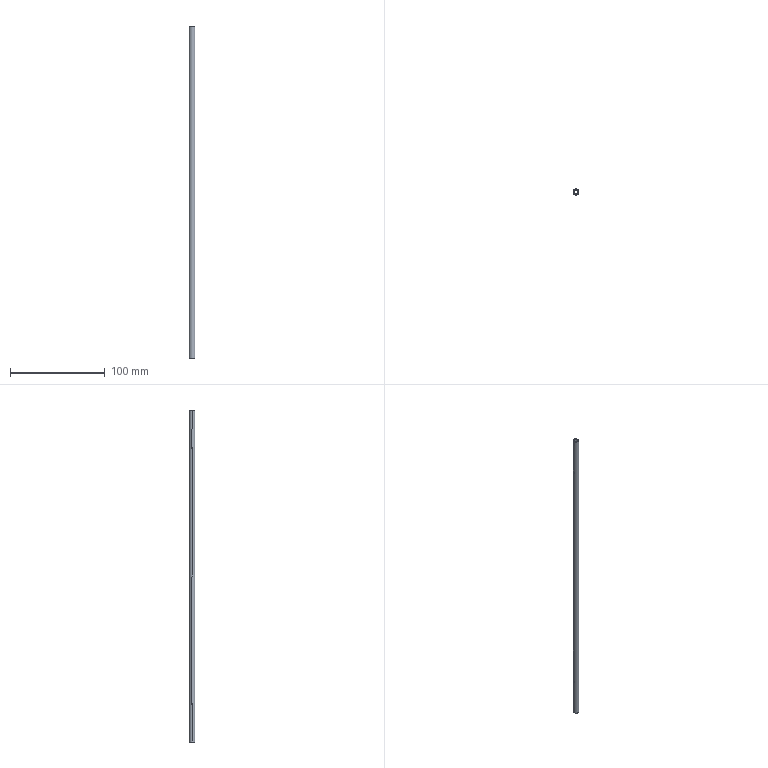Part | SolidWorks | features Extrusion 1, ICE 1 | 1 solid | 14 faces | box 6 x 6 x 350 mm | volume 5491 mm3 | cylinder 12 | plane 2 | commonest cylinder face diameters 1.5 x8 4 x2 6 x2
STEP:
#1=CARTESIAN_POINT('',(-2.,0.,310.75));
#2=VERTEX_POINT('',#1);
#3=CARTESIAN_POINT('',(-2.,0.,309.25));
#4=VERTEX_POINT('',#3);
#5=CARTESIAN_POINT('',(-2.,0.,310.75));
#6=CARTESIAN_POINT('',(-2.,-0.1001,310.75));
#7=CARTESIAN_POINT('',(-1.992,-0.1982,310.73));
#8=CARTESIAN_POINT('',(-1.966,-0.3796,310.654));
#9=CARTESIAN_POINT('',(-1.947,-0.4621,310.599));
#10=CARTESIAN_POINT('',(-1.909,-0.5991,310.461));
#11=CARTESIAN_POINT('',(-1.89,-0.6547,310.379));
#12=CARTESIAN_POINT('',(-1.863,-0.7298,310.199));
#13=CARTESIAN_POINT('',(-1.854,-0.7499,310.099));
#14=CARTESIAN_POINT('',(-1.854,-0.7501,309.902));
#15=CARTESIAN_POINT('',(-1.862,-0.7304,309.803));
#16=CARTESIAN_POINT('',(-1.89,-0.6542,309.62));
#17=CARTESIAN_POINT('',(-1.91,-0.5989,309.538));
#18=CARTESIAN_POINT('',(-1.947,-0.4613,309.401));
#19=CARTESIAN_POINT('',(-1.966,-0.3786,309.345));
#20=CARTESIAN_POINT('',(-1.992,-0.1981,309.27));
#21=CARTESIAN_POINT('',(-2.,-0.09859,309.25));
#22=CARTESIAN_POINT('',(-2.,0.,309.25));
#23=B_SPLINE_CURVE_WITH_KNOTS('',3,(#5,#6,#7,#8,#9,#10,#11,#12,#13,#14,#15,#16,#17,#18,#19,#20,#21,#22),.UNSPECIFIED.,.F.,.F.,(4,2,2,2,2,2,2,2,4),(0.,0.0002958,0.0005917,0.0008875,0.001183,0.001479,0.001775,0.002071,0.002367),.UNSPECIFIED.);
#24=EDGE_CURVE('',#2,#4,#23,.T.);
#25=ORIENTED_EDGE('',*,*,#24,.T.);
#26=CARTESIAN_POINT('',(-3.,0.,309.25));
#27=VERTEX_POINT('',#26);
#28=CARTESIAN_POINT('',(3.,0.,309.25));
#29=DIRECTION('',(-1.,0.,0.));
#30=VECTOR('',#29,1000.);
#31=LINE('',#28,#30);
#32=EDGE_CURVE('',#4,#27,#31,.T.);
#33=ORIENTED_EDGE('',*,*,#32,.T.);
#34=CARTESIAN_POINT('',(-3.,0.,310.75));
#35=VERTEX_POINT('',#34);
#36=CARTESIAN_POINT('',(-3.,0.,310.75));
#37=CARTESIAN_POINT('',(-3.,-0.09953,310.75));
#38=CARTESIAN_POINT('',(-2.995,-0.1972,310.73));
#39=CARTESIAN_POINT('',(-2.977,-0.3787,310.655));
#40=CARTESIAN_POINT('',(-2.965,-0.4616,310.599));
#41=CARTESIAN_POINT('',(-2.94,-0.5994,310.461));
#42=CARTESIAN_POINT('',(-2.928,-0.6552,310.378));
#43=CARTESIAN_POINT('',(-2.91,-0.7301,310.198));
#44=CARTESIAN_POINT('',(-2.905,-0.75,310.099));
#45=CARTESIAN_POINT('',(-2.905,-0.75,309.902));
#46=CARTESIAN_POINT('',(-2.91,-0.7305,309.804));
#47=CARTESIAN_POINT('',(-2.928,-0.6549,309.621));
#48=CARTESIAN_POINT('',(-2.94,-0.5997,309.539));
#49=CARTESIAN_POINT('',(-2.965,-0.4607,309.4));
#50=CARTESIAN_POINT('',(-2.977,-0.3781,309.345));
#51=CARTESIAN_POINT('',(-2.995,-0.197,309.27));
#52=CARTESIAN_POINT('',(-3.,-0.09813,309.25));
#53=CARTESIAN_POINT('',(-3.,0.,309.25));
#54=B_SPLINE_CURVE_WITH_KNOTS('',3,(#36,#37,#38,#39,#40,#41,#42,#43,#44,#45,#46,#47,#48,#49,#50,#51,#52,#53),.UNSPECIFIED.,.F.,.F.,(4,2,2,2,2,2,2,2,4),(0.,0.0002943,0.0005886,0.0008828,0.001177,0.001471,0.001766,0.00206,0.002354),.UNSPECIFIED.);
#55=EDGE_CURVE('',#35,#27,#54,.T.);
#56=ORIENTED_EDGE('',*,*,#55,.F.);
#57=CARTESIAN_POINT('',(3.,0.,310.75));
#58=DIRECTION('',(-1.,0.,0.));
#59=VECTOR('',#58,1000.);
#60=LINE('',#57,#59);
#61=EDGE_CURVE('',#2,#35,#60,.T.);
#62=ORIENTED_EDGE('',*,*,#61,.F.);
#63=EDGE_LOOP('',(#25,#33,#56,#62));
#64=FACE_OUTER_BOUND('',#63,.T.);
#65=CARTESIAN_POINT('',(3.,0.,310.));
#66=DIRECTION('',(-1.,0.,0.));
#67=DIRECTION('',(0.,0.,1.));
#68=AXIS2_PLACEMENT_3D('',#65,#66,#67);
#69=CYLINDRICAL_SURFACE('',#68,0.75);
#70=ADVANCED_FACE('',(#64),#69,.F.);
#71=CARTESIAN_POINT('',(3.,0.,309.25));
#72=VERTEX_POINT('',#71);
#73=CARTESIAN_POINT('',(3.,0.,310.75));
#74=VERTEX_POINT('',#73);
#75=CARTESIAN_POINT('',(3.,0.,309.25));
#76=CARTESIAN_POINT('',(3.,-0.0981,309.25));
#77=CARTESIAN_POINT('',(2.995,-0.1972,309.27));
#78=CARTESIAN_POINT('',(2.977,-0.3778,309.345));
#79=CARTESIAN_POINT('',(2.965,-0.4609,309.4));
#80=CARTESIAN_POINT('',(2.928,-0.6685,309.608));
#81=CARTESIAN_POINT('',(2.905,-0.7499,309.802));
#82=CARTESIAN_POINT('',(2.905,-0.7501,310.198));
#83=CARTESIAN_POINT('',(2.928,-0.6682,310.392));
#84=CARTESIAN_POINT('',(2.977,-0.3931,310.668));
#85=CARTESIAN_POINT('',(3.,-0.199,310.75));
#86=CARTESIAN_POINT('',(3.,0.,310.75));
#87=B_SPLINE_CURVE_WITH_KNOTS('',3,(#75,#76,#77,#78,#79,#80,#81,#82,#83,#84,#85,#86),.UNSPECIFIED.,.F.,.F.,(4,2,2,2,2,4),(0.002354,0.002648,0.002943,0.003531,0.004119,0.004708),.UNSPECIFIED.);
#88=EDGE_CURVE('',#72,#74,#87,.T.);
#89=ORIENTED_EDGE('',*,*,#88,.F.);
#90=CARTESIAN_POINT('',(2.,0.,309.25));
#91=VERTEX_POINT('',#90);
#92=CARTESIAN_POINT('',(3.,0.,309.25));
#93=DIRECTION('',(-1.,0.,0.));
#94=VECTOR('',#93,1000.);
#95=LINE('',#92,#94);
#96=EDGE_CURVE('',#72,#91,#95,.T.);
#97=ORIENTED_EDGE('',*,*,#96,.T.);
#98=CARTESIAN_POINT('',(2.,0.,310.75));
#99=VERTEX_POINT('',#98);
#100=CARTESIAN_POINT('',(2.,0.,309.25));
#101=CARTESIAN_POINT('',(2.,-0.09857,309.25));
#102=CARTESIAN_POINT('',(1.992,-0.198,309.27));
#103=CARTESIAN_POINT('',(1.966,-0.3793,309.346));
#104=CARTESIAN_POINT('',(1.947,-0.4614,309.401));
#105=CARTESIAN_POINT('',(1.909,-0.6,309.539));
#106=CARTESIAN_POINT('',(1.89,-0.6547,309.621));
#107=CARTESIAN_POINT('',(1.862,-0.7302,309.803));
#108=CARTESIAN_POINT('',(1.854,-0.75,309.901));
#109=CARTESIAN_POINT('',(1.854,-0.75,310.099));
#110=CARTESIAN_POINT('',(1.863,-0.7298,310.199));
#111=CARTESIAN_POINT('',(1.89,-0.6545,310.379));
#112=CARTESIAN_POINT('',(1.91,-0.599,310.462));
#113=CARTESIAN_POINT('',(1.947,-0.4614,310.599));
#114=CARTESIAN_POINT('',(1.966,-0.3794,310.654));
#115=CARTESIAN_POINT('',(1.992,-0.1972,310.73));
#116=CARTESIAN_POINT('',(2.,-0.1001,310.75));
#117=CARTESIAN_POINT('',(2.,0.,310.75));
#118=B_SPLINE_CURVE_WITH_KNOTS('',3,(#100,#101,#102,#103,#104,#105,#106,#107,#108,#109,#110,#111,#112,#113,#114,#115,#116,#117),.UNSPECIFIED.,.F.,.F.,(4,2,2,2,2,2,2,2,4),(0.002367,0.002662,0.002958,0.003254,0.00355,0.003846,0.004141,0.004437,0.004733),.UNSPECIFIED.);
#119=EDGE_CURVE('',#91,#99,#118,.T.);
#120=ORIENTED_EDGE('',*,*,#119,.T.);
#121=CARTESIAN_POINT('',(3.,0.,310.75));
#122=DIRECTION('',(-1.,0.,0.));
#123=VECTOR('',#122,1000.);
#124=LINE('',#121,#123);
#125=EDGE_CURVE('',#74,#99,#124,.T.);
#126=ORIENTED_EDGE('',*,*,#125,.F.);
#127=EDGE_LOOP('',(#89,#97,#120,#126));
#128=FACE_OUTER_BOUND('',#127,.T.);
#129=CARTESIAN_POINT('',(3.,0.,310.));
#130=DIRECTION('',(-1.,0.,0.));
#131=DIRECTION('',(0.,0.,1.));
#132=AXIS2_PLACEMENT_3D('',#129,#130,#131);
#133=CYLINDRICAL_SURFACE('',#132,0.75);
#134=ADVANCED_FACE('',(#128),#133,.F.);
#135=CARTESIAN_POINT('',(-2.,0.,40.75));
#136=VERTEX_POINT('',#135);
#137=CARTESIAN_POINT('',(-2.,0.,39.25));
#138=VERTEX_POINT('',#137);
#139=CARTESIAN_POINT('',(-2.,0.,40.75));
#140=CARTESIAN_POINT('',(-2.,-0.1001,40.75));
#141=CARTESIAN_POINT('',(-1.992,-0.1982,40.73));
#142=CARTESIAN_POINT('',(-1.966,-0.3796,40.654));
#143=CARTESIAN_POINT('',(-1.947,-0.4621,40.599));
#144=CARTESIAN_POINT('',(-1.909,-0.5991,40.461));
#145=CARTESIAN_POINT('',(-1.89,-0.6547,40.379));
#146=CARTESIAN_POINT('',(-1.863,-0.7298,40.199));
#147=CARTESIAN_POINT('',(-1.854,-0.7499,40.099));
#148=CARTESIAN_POINT('',(-1.854,-0.7501,39.902));
#149=CARTESIAN_POINT('',(-1.862,-0.7304,39.803));
#150=CARTESIAN_POINT('',(-1.89,-0.6542,39.62));
#151=CARTESIAN_POINT('',(-1.91,-0.5989,39.538));
#152=CARTESIAN_POINT('',(-1.947,-0.4613,39.401));
#153=CARTESIAN_POINT('',(-1.966,-0.3786,39.345));
#154=CARTESIAN_POINT('',(-1.992,-0.1981,39.27));
#155=CARTESIAN_POINT('',(-2.,-0.09859,39.25));
#156=CARTESIAN_POINT('',(-2.,0.,39.25));
#157=B_SPLINE_CURVE_WITH_KNOTS('',3,(#139,#140,#141,#142,#143,#144,#145,#146,#147,#148,#149,#150,#151,#152,#153,#154,#155,#156),.UNSPECIFIED.,.F.,.F.,(4,2,2,2,2,2,2,2,4),(0.,0.0002958,0.0005917,0.0008875,0.001183,0.001479,0.001775,0.002071,0.002367),.UNSPECIFIED.);
#158=EDGE_CURVE('',#136,#138,#157,.T.);
#159=ORIENTED_EDGE('',*,*,#158,.T.);
#160=CARTESIAN_POINT('',(-3.,0.,39.25));
#161=VERTEX_POINT('',#160);
#162=CARTESIAN_POINT('',(3.,0.,39.25));
#163=DIRECTION('',(-1.,0.,0.));
#164=VECTOR('',#163,1000.);
#165=LINE('',#162,#164);
#166=EDGE_CURVE('',#138,#161,#165,.T.);
#167=ORIENTED_EDGE('',*,*,#166,.T.);
#168=CARTESIAN_POINT('',(-3.,0.,40.75));
#169=VERTEX_POINT('',#168);
#170=CARTESIAN_POINT('',(-3.,0.,40.75));
#171=CARTESIAN_POINT('',(-3.,-0.09953,40.75));
#172=CARTESIAN_POINT('',(-2.995,-0.1972,40.73));
#173=CARTESIAN_POINT('',(-2.977,-0.3787,40.655));
#174=CARTESIAN_POINT('',(-2.965,-0.4616,40.599));
#175=CARTESIAN_POINT('',(-2.94,-0.5994,40.461));
#176=CARTESIAN_POINT('',(-2.928,-0.6552,40.378));
#177=CARTESIAN_POINT('',(-2.91,-0.7301,40.198));
#178=CARTESIAN_POINT('',(-2.905,-0.75,40.099));
#179=CARTESIAN_POINT('',(-2.905,-0.75,39.902));
#180=CARTESIAN_POINT('',(-2.91,-0.7305,39.804));
#181=CARTESIAN_POINT('',(-2.928,-0.6549,39.621));
#182=CARTESIAN_POINT('',(-2.94,-0.5997,39.539));
#183=CARTESIAN_POINT('',(-2.965,-0.4607,39.4));
#184=CARTESIAN_POINT('',(-2.977,-0.3781,39.345));
#185=CARTESIAN_POINT('',(-2.995,-0.197,39.27));
#186=CARTESIAN_POINT('',(-3.,-0.09813,39.25));
#187=CARTESIAN_POINT('',(-3.,0.,39.25));
#188=B_SPLINE_CURVE_WITH_KNOTS('',3,(#170,#171,#172,#173,#174,#175,#176,#177,#178,#179,#180,#181,#182,#183,#184,#185,#186,#187),.UNSPECIFIED.,.F.,.F.,(4,2,2,2,2,2,2,2,4),(0.,0.0002943,0.0005886,0.0008828,0.001177,0.001471,0.001766,0.00206,0.002354),.UNSPECIFIED.);
#189=EDGE_CURVE('',#169,#161,#188,.T.);
#190=ORIENTED_EDGE('',*,*,#189,.F.);
#191=CARTESIAN_POINT('',(3.,0.,40.75));
#192=DIRECTION('',(-1.,0.,0.));
#193=VECTOR('',#192,1000.);
#194=LINE('',#191,#193);
#195=EDGE_CURVE('',#136,#169,#194,.T.);
#196=ORIENTED_EDGE('',*,*,#195,.F.);
#197=EDGE_LOOP('',(#159,#167,#190,#196));
#198=FACE_OUTER_BOUND('',#197,.T.);
#199=CARTESIAN_POINT('',(3.,0.,40.));
#200=DIRECTION('',(-1.,0.,0.));
#201=DIRECTION('',(0.,0.,1.));
#202=AXIS2_PLACEMENT_3D('',#199,#200,#201);
#203=CYLINDRICAL_SURFACE('',#202,0.75);
#204=ADVANCED_FACE('',(#198),#203,.F.);
#205=CARTESIAN_POINT('',(3.,0.,39.25));
#206=VERTEX_POINT('',#205);
#207=CARTESIAN_POINT('',(3.,0.,40.75));
#208=VERTEX_POINT('',#207);
#209=CARTESIAN_POINT('',(3.,0.,39.25));
#210=CARTESIAN_POINT('',(3.,-0.0981,39.25));
#211=CARTESIAN_POINT('',(2.995,-0.1972,39.27));
#212=CARTESIAN_POINT('',(2.977,-0.3778,39.345));
#213=CARTESIAN_POINT('',(2.965,-0.4609,39.4));
#214=CARTESIAN_POINT('',(2.928,-0.6685,39.608));
#215=CARTESIAN_POINT('',(2.905,-0.7499,39.802));
#216=CARTESIAN_POINT('',(2.905,-0.7501,40.198));
#217=CARTESIAN_POINT('',(2.928,-0.6682,40.392));
#218=CARTESIAN_POINT('',(2.977,-0.3931,40.668));
#219=CARTESIAN_POINT('',(3.,-0.199,40.75));
#220=CARTESIAN_POINT('',(3.,0.,40.75));
#221=B_SPLINE_CURVE_WITH_KNOTS('',3,(#209,#210,#211,#212,#213,#214,#215,#216,#217,#218,#219,#220),.UNSPECIFIED.,.F.,.F.,(4,2,2,2,2,4),(0.002354,0.002648,0.002943,0.003531,0.004119,0.004708),.UNSPECIFIED.);
#222=EDGE_CURVE('',#206,#208,#221,.T.);
#223=ORIENTED_EDGE('',*,*,#222,.F.);
#224=CARTESIAN_POINT('',(2.,0.,39.25));
#225=VERTEX_POINT('',#224);
#226=CARTESIAN_POINT('',(3.,0.,39.25));
#227=DIRECTION('',(-1.,0.,0.));
#228=VECTOR('',#227,1000.);
#229=LINE('',#226,#228);
#230=EDGE_CURVE('',#206,#225,#229,.T.);
#231=ORIENTED_EDGE('',*,*,#230,.T.);
#232=CARTESIAN_POINT('',(2.,0.,40.75));
#233=VERTEX_POINT('',#232);
#234=CARTESIAN_POINT('',(2.,0.,39.25));
#235=CARTESIAN_POINT('',(2.,-0.09857,39.25));
#236=CARTESIAN_POINT('',(1.992,-0.198,39.27));
#237=CARTESIAN_POINT('',(1.966,-0.3793,39.346));
#238=CARTESIAN_POINT('',(1.947,-0.4614,39.401));
#239=CARTESIAN_POINT('',(1.909,-0.6,39.539));
#240=CARTESIAN_POINT('',(1.89,-0.6547,39.621));
#241=CARTESIAN_POINT('',(1.862,-0.7302,39.803));
#242=CARTESIAN_POINT('',(1.854,-0.75,39.901));
#243=CARTESIAN_POINT('',(1.854,-0.75,40.099));
#244=CARTESIAN_POINT('',(1.863,-0.7298,40.199));
#245=CARTESIAN_POINT('',(1.89,-0.6545,40.379));
#246=CARTESIAN_POINT('',(1.91,-0.599,40.462));
#247=CARTESIAN_POINT('',(1.947,-0.4614,40.599));
#248=CARTESIAN_POINT('',(1.966,-0.3794,40.654));
#249=CARTESIAN_POINT('',(1.992,-0.1972,40.73));
#250=CARTESIAN_POINT('',(2.,-0.1001,40.75));
#251=CARTESIAN_POINT('',(2.,0.,40.75));
#252=B_SPLINE_CURVE_WITH_KNOTS('',3,(#234,#235,#236,#237,#238,#239,#240,#241,#242,#243,#244,#245,#246,#247,#248,#249,#250,#251),.UNSPECIFIED.,.F.,.F.,(4,2,2,2,2,2,2,2,4),(0.002367,0.002662,0.002958,0.003254,0.00355,0.003846,0.004141,0.004437,0.004733),.UNSPECIFIED.);
#253=EDGE_CURVE('',#225,#233,#252,.T.);
#254=ORIENTED_EDGE('',*,*,#253,.T.);
#255=CARTESIAN_POINT('',(3.,0.,40.75));
#256=DIRECTION('',(-1.,0.,0.));
#257=VECTOR('',#256,1000.);
#258=LINE('',#255,#257);
#259=EDGE_CURVE('',#208,#233,#258,.T.);
#260=ORIENTED_EDGE('',*,*,#259,.F.);
#261=EDGE_LOOP('',(#223,#231,#254,#260));
#262=FACE_OUTER_BOUND('',#261,.T.);
#263=CARTESIAN_POINT('',(3.,0.,40.));
#264=DIRECTION('',(-1.,0.,0.));
#265=DIRECTION('',(0.,0.,1.));
#266=AXIS2_PLACEMENT_3D('',#263,#264,#265);
#267=CYLINDRICAL_SURFACE('',#266,0.75);
#268=ADVANCED_FACE('',(#262),#267,.F.);
#269=CARTESIAN_POINT('',(-2.,0.,350.));
#270=VERTEX_POINT('',#269);
#271=CARTESIAN_POINT('',(2.,0.,350.));
#272=VERTEX_POINT('',#271);
#273=CARTESIAN_POINT('',(0.,0.,350.));
#274=DIRECTION('',(0.,0.,1.));
#275=DIRECTION('',(1.,0.,0.));
#276=AXIS2_PLACEMENT_3D('',#273,#274,#275);
#277=CIRCLE('',#276,2.);
#278=EDGE_CURVE('',#270,#272,#277,.T.);
#279=ORIENTED_EDGE('',*,*,#278,.T.);
#280=CARTESIAN_POINT('',(2.,0.,350.));
#281=DIRECTION('',(0.,0.,-1.));
#282=VECTOR('',#281,1000.);
#283=LINE('',#280,#282);
#284=EDGE_CURVE('',#272,#99,#283,.T.);
#285=ORIENTED_EDGE('',*,*,#284,.T.);
#286=ORIENTED_EDGE('',*,*,#119,.F.);
#287=CARTESIAN_POINT('',(2.,0.,350.));
#288=DIRECTION('',(0.,0.,-1.));
#289=VECTOR('',#288,1000.);
#290=LINE('',#287,#289);
#291=EDGE_CURVE('',#91,#233,#290,.T.);
#292=ORIENTED_EDGE('',*,*,#291,.T.);
#293=ORIENTED_EDGE('',*,*,#253,.F.);
#294=CARTESIAN_POINT('',(2.,0.,0.));
#295=VERTEX_POINT('',#294);
#296=CARTESIAN_POINT('',(2.,0.,350.));
#297=DIRECTION('',(0.,0.,-1.));
#298=VECTOR('',#297,1000.);
#299=LINE('',#296,#298);
#300=EDGE_CURVE('',#225,#295,#299,.T.);
#301=ORIENTED_EDGE('',*,*,#300,.T.);
#302=CARTESIAN_POINT('',(-2.,0.,0.));
#303=VERTEX_POINT('',#302);
#304=CARTESIAN_POINT('',(0.,0.,0.));
#305=DIRECTION('',(0.,0.,1.));
#306=DIRECTION('',(1.,0.,0.));
#307=AXIS2_PLACEMENT_3D('',#304,#305,#306);
#308=CIRCLE('',#307,2.);
#309=EDGE_CURVE('',#303,#295,#308,.T.);
#310=ORIENTED_EDGE('',*,*,#309,.F.);
#311=CARTESIAN_POINT('',(-2.,0.,350.));
#312=DIRECTION('',(0.,0.,-1.));
#313=VECTOR('',#312,1000.);
#314=LINE('',#311,#313);
#315=EDGE_CURVE('',#138,#303,#314,.T.);
#316=ORIENTED_EDGE('',*,*,#315,.F.);
#317=ORIENTED_EDGE('',*,*,#158,.F.);
#318=CARTESIAN_POINT('',(-2.,0.,350.));
#319=DIRECTION('',(0.,0.,-1.));
#320=VECTOR('',#319,1000.);
#321=LINE('',#318,#320);
#322=EDGE_CURVE('',#4,#136,#321,.T.);
#323=ORIENTED_EDGE('',*,*,#322,.F.);
#324=ORIENTED_EDGE('',*,*,#24,.F.);
#325=CARTESIAN_POINT('',(-2.,0.,350.));
#326=DIRECTION('',(0.,0.,-1.));
#327=VECTOR('',#326,1000.);
#328=LINE('',#325,#327);
#329=EDGE_CURVE('',#270,#2,#328,.T.);
#330=ORIENTED_EDGE('',*,*,#329,.F.);
#331=EDGE_LOOP('',(#279,#285,#286,#292,#293,#301,#310,#316,#317,#323,#324,#330));
#332=FACE_OUTER_BOUND('',#331,.T.);
#333=CARTESIAN_POINT('',(0.,0.,350.));
#334=DIRECTION('',(0.,0.,-1.));
#335=DIRECTION('',(-1.,0.,0.));
#336=AXIS2_PLACEMENT_3D('',#333,#334,#335);
#337=CYLINDRICAL_SURFACE('',#336,2.);
#338=ADVANCED_FACE('',(#332),#337,.F.);
#339=CARTESIAN_POINT('',(3.,0.,350.));
#340=VERTEX_POINT('',#339);
#341=CARTESIAN_POINT('',(-3.,0.,350.));
#342=VERTEX_POINT('',#341);
#343=CARTESIAN_POINT('',(0.,0.,350.));
#344=DIRECTION('',(0.,0.,1.));
#345=DIRECTION('',(1.,0.,0.));
#346=AXIS2_PLACEMENT_3D('',#343,#344,#345);
#347=CIRCLE('',#346,3.);
#348=EDGE_CURVE('',#340,#342,#347,.T.);
#349=ORIENTED_EDGE('',*,*,#348,.F.);
#350=CARTESIAN_POINT('',(3.,0.,350.));
#351=DIRECTION('',(0.,0.,-1.));
#352=VECTOR('',#351,1000.);
#353=LINE('',#350,#352);
#354=EDGE_CURVE('',#340,#74,#353,.T.);
#355=ORIENTED_EDGE('',*,*,#354,.T.);
#356=CARTESIAN_POINT('',(3.,0.,310.75));
#357=CARTESIAN_POINT('',(3.,0.09953,310.75));
#358=CARTESIAN_POINT('',(2.995,0.1972,310.73));
#359=CARTESIAN_POINT('',(2.977,0.3787,310.655));
#360=CARTESIAN_POINT('',(2.965,0.4616,310.599));
#361=CARTESIAN_POINT('',(2.94,0.5994,310.461));
#362=CARTESIAN_POINT('',(2.928,0.6552,310.378));
#363=CARTESIAN_POINT('',(2.91,0.7301,310.198));
#364=CARTESIAN_POINT('',(2.905,0.75,310.099));
#365=CARTESIAN_POINT('',(2.905,0.75,309.902));
#366=CARTESIAN_POINT('',(2.91,0.7305,309.804));
#367=CARTESIAN_POINT('',(2.928,0.6549,309.621));
#368=CARTESIAN_POINT('',(2.94,0.5997,309.539));
#369=CARTESIAN_POINT('',(2.965,0.4607,309.4));
#370=CARTESIAN_POINT('',(2.977,0.3781,309.345));
#371=CARTESIAN_POINT('',(2.995,0.197,309.27));
#372=CARTESIAN_POINT('',(3.,0.09813,309.25));
#373=CARTESIAN_POINT('',(3.,0.,309.25));
#374=B_SPLINE_CURVE_WITH_KNOTS('',3,(#356,#357,#358,#359,#360,#361,#362,#363,#364,#365,#366,#367,#368,#369,#370,#371,#372,#373),.UNSPECIFIED.,.F.,.F.,(4,2,2,2,2,2,2,2,4),(0.,0.0002943,0.0005886,0.0008828,0.001177,0.001471,0.001766,0.00206,0.002354),.UNSPECIFIED.);
#375=EDGE_CURVE('',#74,#72,#374,.T.);
#376=ORIENTED_EDGE('',*,*,#375,.T.);
#377=CARTESIAN_POINT('',(3.,0.,350.));
#378=DIRECTION('',(0.,0.,-1.));
#379=VECTOR('',#378,1000.);
#380=LINE('',#377,#379);
#381=EDGE_CURVE('',#72,#208,#380,.T.);
#382=ORIENTED_EDGE('',*,*,#381,.T.);
#383=CARTESIAN_POINT('',(3.,0.,40.75));
#384=CARTESIAN_POINT('',(3.,0.09953,40.75));
#385=CARTESIAN_POINT('',(2.995,0.1972,40.73));
#386=CARTESIAN_POINT('',(2.977,0.3787,40.655));
#387=CARTESIAN_POINT('',(2.965,0.4616,40.599));
#388=CARTESIAN_POINT('',(2.94,0.5994,40.461));
#389=CARTESIAN_POINT('',(2.928,0.6552,40.378));
#390=CARTESIAN_POINT('',(2.91,0.7301,40.198));
#391=CARTESIAN_POINT('',(2.905,0.75,40.099));
#392=CARTESIAN_POINT('',(2.905,0.75,39.902));
#393=CARTESIAN_POINT('',(2.91,0.7305,39.804));
#394=CARTESIAN_POINT('',(2.928,0.6549,39.621));
#395=CARTESIAN_POINT('',(2.94,0.5997,39.539));
#396=CARTESIAN_POINT('',(2.965,0.4607,39.4));
#397=CARTESIAN_POINT('',(2.977,0.3781,39.345));
#398=CARTESIAN_POINT('',(2.995,0.197,39.27));
#399=CARTESIAN_POINT('',(3.,0.09813,39.25));
#400=CARTESIAN_POINT('',(3.,0.,39.25));
#401=B_SPLINE_CURVE_WITH_KNOTS('',3,(#383,#384,#385,#386,#387,#388,#389,#390,#391,#392,#393,#394,#395,#396,#397,#398,#399,#400),.UNSPECIFIED.,.F.,.F.,(4,2,2,2,2,2,2,2,4),(0.,0.0002943,0.0005886,0.0008828,0.001177,0.001471,0.001766,0.00206,0.002354),.UNSPECIFIED.);
#402=EDGE_CURVE('',#208,#206,#401,.T.);
#403=ORIENTED_EDGE('',*,*,#402,.T.);
#404=CARTESIAN_POINT('',(3.,0.,0.));
#405=VERTEX_POINT('',#404);
#406=CARTESIAN_POINT('',(3.,0.,350.));
#407=DIRECTION('',(0.,0.,-1.));
#408=VECTOR('',#407,1000.);
#409=LINE('',#406,#408);
#410=EDGE_CURVE('',#206,#405,#409,.T.);
#411=ORIENTED_EDGE('',*,*,#410,.T.);
#412=CARTESIAN_POINT('',(-3.,0.,0.));
#413=VERTEX_POINT('',#412);
#414=CARTESIAN_POINT('',(0.,0.,0.));
#415=DIRECTION('',(0.,0.,1.));
#416=DIRECTION('',(1.,0.,0.));
#417=AXIS2_PLACEMENT_3D('',#414,#415,#416);
#418=CIRCLE('',#417,3.);
#419=EDGE_CURVE('',#405,#413,#418,.T.);
#420=ORIENTED_EDGE('',*,*,#419,.T.);
#421=CARTESIAN_POINT('',(-3.,0.,350.));
#422=DIRECTION('',(0.,0.,-1.));
#423=VECTOR('',#422,1000.);
#424=LINE('',#421,#423);
#425=EDGE_CURVE('',#161,#413,#424,.T.);
#426=ORIENTED_EDGE('',*,*,#425,.F.);
#427=CARTESIAN_POINT('',(-3.,0.,39.25));
#428=CARTESIAN_POINT('',(-3.,0.0981,39.25));
#429=CARTESIAN_POINT('',(-2.995,0.1972,39.27));
#430=CARTESIAN_POINT('',(-2.977,0.3778,39.345));
#431=CARTESIAN_POINT('',(-2.965,0.4609,39.4));
#432=CARTESIAN_POINT('',(-2.928,0.6685,39.608));
#433=CARTESIAN_POINT('',(-2.905,0.7499,39.802));
#434=CARTESIAN_POINT('',(-2.905,0.7501,40.198));
#435=CARTESIAN_POINT('',(-2.928,0.6682,40.392));
#436=CARTESIAN_POINT('',(-2.977,0.3931,40.668));
#437=CARTESIAN_POINT('',(-3.,0.199,40.75));
#438=CARTESIAN_POINT('',(-3.,0.,40.75));
#439=B_SPLINE_CURVE_WITH_KNOTS('',3,(#427,#428,#429,#430,#431,#432,#433,#434,#435,#436,#437,#438),.UNSPECIFIED.,.F.,.F.,(4,2,2,2,2,4),(0.002354,0.002648,0.002943,0.003531,0.004119,0.004708),.UNSPECIFIED.);
#440=EDGE_CURVE('',#161,#169,#439,.T.);
#441=ORIENTED_EDGE('',*,*,#440,.T.);
#442=CARTESIAN_POINT('',(-3.,0.,350.));
#443=DIRECTION('',(0.,0.,-1.));
#444=VECTOR('',#443,1000.);
#445=LINE('',#442,#444);
#446=EDGE_CURVE('',#27,#169,#445,.T.);
#447=ORIENTED_EDGE('',*,*,#446,.F.);
#448=CARTESIAN_POINT('',(-3.,0.,309.25));
#449=CARTESIAN_POINT('',(-3.,0.0981,309.25));
#450=CARTESIAN_POINT('',(-2.995,0.1972,309.27));
#451=CARTESIAN_POINT('',(-2.977,0.3778,309.345));
#452=CARTESIAN_POINT('',(-2.965,0.4609,309.4));
#453=CARTESIAN_POINT('',(-2.928,0.6685,309.608));
#454=CARTESIAN_POINT('',(-2.905,0.7499,309.802));
#455=CARTESIAN_POINT('',(-2.905,0.7501,310.198));
#456=CARTESIAN_POINT('',(-2.928,0.6682,310.392));
#457=CARTESIAN_POINT('',(-2.977,0.3931,310.668));
#458=CARTESIAN_POINT('',(-3.,0.199,310.75));
#459=CARTESIAN_POINT('',(-3.,0.,310.75));
#460=B_SPLINE_CURVE_WITH_KNOTS('',3,(#448,#449,#450,#451,#452,#453,#454,#455,#456,#457,#458,#459),.UNSPECIFIED.,.F.,.F.,(4,2,2,2,2,4),(0.002354,0.002648,0.002943,0.003531,0.004119,0.004708),.UNSPECIFIED.);
#461=EDGE_CURVE('',#27,#35,#460,.T.);
#462=ORIENTED_EDGE('',*,*,#461,.T.);
#463=CARTESIAN_POINT('',(-3.,0.,350.));
#464=DIRECTION('',(0.,0.,-1.));
#465=VECTOR('',#464,1000.);
#466=LINE('',#463,#465);
#467=EDGE_CURVE('',#342,#35,#466,.T.);
#468=ORIENTED_EDGE('',*,*,#467,.F.);
#469=EDGE_LOOP('',(#349,#355,#376,#382,#403,#411,#420,#426,#441,#447,#462,#468));
#470=FACE_OUTER_BOUND('',#469,.T.);
#471=CARTESIAN_POINT('',(0.,0.,350.));
#472=DIRECTION('',(0.,0.,-1.));
#473=DIRECTION('',(-1.,0.,0.));
#474=AXIS2_PLACEMENT_3D('',#471,#472,#473);
#475=CYLINDRICAL_SURFACE('',#474,3.);
#476=ADVANCED_FACE('',(#470),#475,.T.);
#477=CARTESIAN_POINT('',(0.,0.,350.));
#478=DIRECTION('',(0.,0.,1.));
#479=DIRECTION('',(1.,0.,0.));
#480=AXIS2_PLACEMENT_3D('',#477,#478,#479);
#481=CIRCLE('',#480,3.);
#482=EDGE_CURVE('',#342,#340,#481,.T.);
#483=ORIENTED_EDGE('',*,*,#482,.T.);
#484=ORIENTED_EDGE('',*,*,#348,.T.);
#485=EDGE_LOOP('',(#483,#484));
#486=FACE_OUTER_BOUND('',#485,.T.);
#487=ORIENTED_EDGE('',*,*,#278,.F.);
#488=CARTESIAN_POINT('',(0.,0.,350.));
#489=DIRECTION('',(0.,0.,1.));
#490=DIRECTION('',(1.,0.,0.));
#491=AXIS2_PLACEMENT_3D('',#488,#489,#490);
#492=CIRCLE('',#491,2.);
#493=EDGE_CURVE('',#272,#270,#492,.T.);
#494=ORIENTED_EDGE('',*,*,#493,.F.);
#495=EDGE_LOOP('',(#487,#494));
#496=FACE_BOUND('',#495,.T.);
#497=CARTESIAN_POINT('',(0.,0.,350.));
#498=DIRECTION('',(0.,0.,1.));
#499=DIRECTION('',(1.,0.,0.));
#500=AXIS2_PLACEMENT_3D('',#497,#498,#499);
#501=PLANE('',#500);
#502=ADVANCED_FACE('',(#486,#496),#501,.T.);
#503=CARTESIAN_POINT('',(0.,0.,0.));
#504=DIRECTION('',(0.,0.,1.));
#505=DIRECTION('',(1.,0.,0.));
#506=AXIS2_PLACEMENT_3D('',#503,#504,#505);
#507=CIRCLE('',#506,3.);
#508=EDGE_CURVE('',#413,#405,#507,.T.);
#509=ORIENTED_EDGE('',*,*,#508,.F.);
#510=ORIENTED_EDGE('',*,*,#419,.F.);
#511=EDGE_LOOP('',(#509,#510));
#512=FACE_OUTER_BOUND('',#511,.T.);
#513=ORIENTED_EDGE('',*,*,#309,.T.);
#514=CARTESIAN_POINT('',(0.,0.,0.));
#515=DIRECTION('',(0.,0.,1.));
#516=DIRECTION('',(1.,0.,0.));
#517=AXIS2_PLACEMENT_3D('',#514,#515,#516);
#518=CIRCLE('',#517,2.);
#519=EDGE_CURVE('',#295,#303,#518,.T.);
#520=ORIENTED_EDGE('',*,*,#519,.T.);
#521=EDGE_LOOP('',(#513,#520));
#522=FACE_BOUND('',#521,.T.);
#523=CARTESIAN_POINT('',(0.,0.,0.));
#524=DIRECTION('',(0.,0.,1.));
#525=DIRECTION('',(1.,0.,0.));
#526=AXIS2_PLACEMENT_3D('',#523,#524,#525);
#527=PLANE('',#526);
#528=ADVANCED_FACE('',(#512,#522),#527,.F.);
#529=ORIENTED_EDGE('',*,*,#354,.F.);
#530=ORIENTED_EDGE('',*,*,#482,.F.);
#531=ORIENTED_EDGE('',*,*,#467,.T.);
#532=ORIENTED_EDGE('',*,*,#55,.T.);
#533=ORIENTED_EDGE('',*,*,#446,.T.);
#534=ORIENTED_EDGE('',*,*,#189,.T.);
#535=ORIENTED_EDGE('',*,*,#425,.T.);
#536=ORIENTED_EDGE('',*,*,#508,.T.);
#537=ORIENTED_EDGE('',*,*,#410,.F.);
#538=ORIENTED_EDGE('',*,*,#222,.T.);
#539=ORIENTED_EDGE('',*,*,#381,.F.);
#540=ORIENTED_EDGE('',*,*,#88,.T.);
#541=EDGE_LOOP('',(#529,#530,#531,#532,#533,#534,#535,#536,#537,#538,#539,#540));
#542=FACE_OUTER_BOUND('',#541,.T.);
#543=CARTESIAN_POINT('',(0.,0.,350.));
#544=DIRECTION('',(0.,0.,-1.));
#545=DIRECTION('',(-1.,0.,0.));
#546=AXIS2_PLACEMENT_3D('',#543,#544,#545);
#547=CYLINDRICAL_SURFACE('',#546,3.);
#548=ADVANCED_FACE('',(#542),#547,.T.);
#549=ORIENTED_EDGE('',*,*,#284,.F.);
#550=ORIENTED_EDGE('',*,*,#493,.T.);
#551=ORIENTED_EDGE('',*,*,#329,.T.);
#552=CARTESIAN_POINT('',(-2.,0.,309.25));
#553=CARTESIAN_POINT('',(-2.,0.09857,309.25));
#554=CARTESIAN_POINT('',(-1.992,0.198,309.27));
#555=CARTESIAN_POINT('',(-1.966,0.3793,309.346));
#556=CARTESIAN_POINT('',(-1.947,0.4614,309.401));
#557=CARTESIAN_POINT('',(-1.909,0.6,309.539));
#558=CARTESIAN_POINT('',(-1.89,0.6547,309.621));
#559=CARTESIAN_POINT('',(-1.862,0.7302,309.803));
#560=CARTESIAN_POINT('',(-1.854,0.75,309.901));
#561=CARTESIAN_POINT('',(-1.854,0.75,310.099));
#562=CARTESIAN_POINT('',(-1.863,0.7298,310.199));
#563=CARTESIAN_POINT('',(-1.89,0.6545,310.379));
#564=CARTESIAN_POINT('',(-1.91,0.599,310.462));
#565=CARTESIAN_POINT('',(-1.947,0.4614,310.599));
#566=CARTESIAN_POINT('',(-1.966,0.3794,310.654));
#567=CARTESIAN_POINT('',(-1.992,0.1972,310.73));
#568=CARTESIAN_POINT('',(-2.,0.1001,310.75));
#569=CARTESIAN_POINT('',(-2.,0.,310.75));
#570=B_SPLINE_CURVE_WITH_KNOTS('',3,(#552,#553,#554,#555,#556,#557,#558,#559,#560,#561,#562,#563,#564,#565,#566,#567,#568,#569),.UNSPECIFIED.,.F.,.F.,(4,2,2,2,2,2,2,2,4),(0.002367,0.002662,0.002958,0.003254,0.00355,0.003846,0.004141,0.004437,0.004733),.UNSPECIFIED.);
#571=EDGE_CURVE('',#4,#2,#570,.T.);
#572=ORIENTED_EDGE('',*,*,#571,.F.);
#573=ORIENTED_EDGE('',*,*,#322,.T.);
#574=CARTESIAN_POINT('',(-2.,0.,39.25));
#575=CARTESIAN_POINT('',(-2.,0.09857,39.25));
#576=CARTESIAN_POINT('',(-1.992,0.198,39.27));
#577=CARTESIAN_POINT('',(-1.966,0.3793,39.346));
#578=CARTESIAN_POINT('',(-1.947,0.4614,39.401));
#579=CARTESIAN_POINT('',(-1.909,0.6,39.539));
#580=CARTESIAN_POINT('',(-1.89,0.6547,39.621));
#581=CARTESIAN_POINT('',(-1.862,0.7302,39.803));
#582=CARTESIAN_POINT('',(-1.854,0.75,39.901));
#583=CARTESIAN_POINT('',(-1.854,0.75,40.099));
#584=CARTESIAN_POINT('',(-1.863,0.7298,40.199));
#585=CARTESIAN_POINT('',(-1.89,0.6545,40.379));
#586=CARTESIAN_POINT('',(-1.91,0.599,40.462));
#587=CARTESIAN_POINT('',(-1.947,0.4614,40.599));
#588=CARTESIAN_POINT('',(-1.966,0.3794,40.654));
#589=CARTESIAN_POINT('',(-1.992,0.1972,40.73));
#590=CARTESIAN_POINT('',(-2.,0.1001,40.75));
#591=CARTESIAN_POINT('',(-2.,0.,40.75));
#592=B_SPLINE_CURVE_WITH_KNOTS('',3,(#574,#575,#576,#577,#578,#579,#580,#581,#582,#583,#584,#585,#586,#587,#588,#589,#590,#591),.UNSPECIFIED.,.F.,.F.,(4,2,2,2,2,2,2,2,4),(0.002367,0.002662,0.002958,0.003254,0.00355,0.003846,0.004141,0.004437,0.004733),.UNSPECIFIED.);
#593=EDGE_CURVE('',#138,#136,#592,.T.);
#594=ORIENTED_EDGE('',*,*,#593,.F.);
#595=ORIENTED_EDGE('',*,*,#315,.T.);
#596=ORIENTED_EDGE('',*,*,#519,.F.);
#597=ORIENTED_EDGE('',*,*,#300,.F.);
#598=CARTESIAN_POINT('',(2.,0.,40.75));
#599=CARTESIAN_POINT('',(2.,0.1001,40.75));
#600=CARTESIAN_POINT('',(1.992,0.1982,40.73));
#601=CARTESIAN_POINT('',(1.966,0.3796,40.654));
#602=CARTESIAN_POINT('',(1.947,0.4621,40.599));
#603=CARTESIAN_POINT('',(1.909,0.5991,40.461));
#604=CARTESIAN_POINT('',(1.89,0.6547,40.379));
#605=CARTESIAN_POINT('',(1.863,0.7298,40.199));
#606=CARTESIAN_POINT('',(1.854,0.7499,40.099));
#607=CARTESIAN_POINT('',(1.854,0.7501,39.902));
#608=CARTESIAN_POINT('',(1.862,0.7304,39.803));
#609=CARTESIAN_POINT('',(1.89,0.6542,39.62));
#610=CARTESIAN_POINT('',(1.91,0.5989,39.538));
#611=CARTESIAN_POINT('',(1.947,0.4613,39.401));
#612=CARTESIAN_POINT('',(1.966,0.3786,39.345));
#613=CARTESIAN_POINT('',(1.992,0.1981,39.27));
#614=CARTESIAN_POINT('',(2.,0.09859,39.25));
#615=CARTESIAN_POINT('',(2.,0.,39.25));
#616=B_SPLINE_CURVE_WITH_KNOTS('',3,(#598,#599,#600,#601,#602,#603,#604,#605,#606,#607,#608,#609,#610,#611,#612,#613,#614,#615),.UNSPECIFIED.,.F.,.F.,(4,2,2,2,2,2,2,2,4),(0.,0.0002958,0.0005917,0.0008875,0.001183,0.001479,0.001775,0.002071,0.002367),.UNSPECIFIED.);
#617=EDGE_CURVE('',#233,#225,#616,.T.);
#618=ORIENTED_EDGE('',*,*,#617,.F.);
#619=ORIENTED_EDGE('',*,*,#291,.F.);
#620=CARTESIAN_POINT('',(2.,0.,310.75));
#621=CARTESIAN_POINT('',(2.,0.1001,310.75));
#622=CARTESIAN_POINT('',(1.992,0.1982,310.73));
#623=CARTESIAN_POINT('',(1.966,0.3796,310.654));
#624=CARTESIAN_POINT('',(1.947,0.4621,310.599));
#625=CARTESIAN_POINT('',(1.909,0.5991,310.461));
#626=CARTESIAN_POINT('',(1.89,0.6547,310.379));
#627=CARTESIAN_POINT('',(1.863,0.7298,310.199));
#628=CARTESIAN_POINT('',(1.854,0.7499,310.099));
#629=CARTESIAN_POINT('',(1.854,0.7501,309.902));
#630=CARTESIAN_POINT('',(1.862,0.7304,309.803));
#631=CARTESIAN_POINT('',(1.89,0.6542,309.62));
#632=CARTESIAN_POINT('',(1.91,0.5989,309.538));
#633=CARTESIAN_POINT('',(1.947,0.4613,309.401));
#634=CARTESIAN_POINT('',(1.966,0.3786,309.345));
#635=CARTESIAN_POINT('',(1.992,0.1981,309.27));
#636=CARTESIAN_POINT('',(2.,0.09859,309.25));
#637=CARTESIAN_POINT('',(2.,0.,309.25));
#638=B_SPLINE_CURVE_WITH_KNOTS('',3,(#620,#621,#622,#623,#624,#625,#626,#627,#628,#629,#630,#631,#632,#633,#634,#635,#636,#637),.UNSPECIFIED.,.F.,.F.,(4,2,2,2,2,2,2,2,4),(0.,0.0002958,0.0005917,0.0008875,0.001183,0.001479,0.001775,0.002071,0.002367),.UNSPECIFIED.);
#639=EDGE_CURVE('',#99,#91,#638,.T.);
#640=ORIENTED_EDGE('',*,*,#639,.F.);
#641=EDGE_LOOP('',(#549,#550,#551,#572,#573,#594,#595,#596,#597,#618,#619,#640));
#642=FACE_OUTER_BOUND('',#641,.T.);
#643=CARTESIAN_POINT('',(0.,0.,350.));
#644=DIRECTION('',(0.,0.,-1.));
#645=DIRECTION('',(-1.,0.,0.));
#646=AXIS2_PLACEMENT_3D('',#643,#644,#645);
#647=CYLINDRICAL_SURFACE('',#646,2.);
#648=ADVANCED_FACE('',(#642),#647,.F.);
#649=ORIENTED_EDGE('',*,*,#230,.F.);
#650=ORIENTED_EDGE('',*,*,#402,.F.);
#651=ORIENTED_EDGE('',*,*,#259,.T.);
#652=ORIENTED_EDGE('',*,*,#617,.T.);
#653=EDGE_LOOP('',(#649,#650,#651,#652));
#654=FACE_OUTER_BOUND('',#653,.T.);
#655=CARTESIAN_POINT('',(3.,0.,40.));
#656=DIRECTION('',(-1.,0.,0.));
#657=DIRECTION('',(0.,0.,1.));
#658=AXIS2_PLACEMENT_3D('',#655,#656,#657);
#659=CYLINDRICAL_SURFACE('',#658,0.75);
#660=ADVANCED_FACE('',(#654),#659,.F.);
#661=ORIENTED_EDGE('',*,*,#166,.F.);
#662=ORIENTED_EDGE('',*,*,#593,.T.);
#663=ORIENTED_EDGE('',*,*,#195,.T.);
#664=ORIENTED_EDGE('',*,*,#440,.F.);
#665=EDGE_LOOP('',(#661,#662,#663,#664));
#666=FACE_OUTER_BOUND('',#665,.T.);
#667=CARTESIAN_POINT('',(3.,0.,40.));
#668=DIRECTION('',(-1.,0.,0.));
#669=DIRECTION('',(0.,0.,1.));
#670=AXIS2_PLACEMENT_3D('',#667,#668,#669);
#671=CYLINDRICAL_SURFACE('',#670,0.75);
#672=ADVANCED_FACE('',(#666),#671,.F.);
#673=ORIENTED_EDGE('',*,*,#96,.F.);
#674=ORIENTED_EDGE('',*,*,#375,.F.);
#675=ORIENTED_EDGE('',*,*,#125,.T.);
#676=ORIENTED_EDGE('',*,*,#639,.T.);
#677=EDGE_LOOP('',(#673,#674,#675,#676));
#678=FACE_OUTER_BOUND('',#677,.T.);
#679=CARTESIAN_POINT('',(3.,0.,310.));
#680=DIRECTION('',(-1.,0.,0.));
#681=DIRECTION('',(0.,0.,1.));
#682=AXIS2_PLACEMENT_3D('',#679,#680,#681);
#683=CYLINDRICAL_SURFACE('',#682,0.75);
#684=ADVANCED_FACE('',(#678),#683,.F.);
#685=ORIENTED_EDGE('',*,*,#32,.F.);
#686=ORIENTED_EDGE('',*,*,#571,.T.);
#687=ORIENTED_EDGE('',*,*,#61,.T.);
#688=ORIENTED_EDGE('',*,*,#461,.F.);
#689=EDGE_LOOP('',(#685,#686,#687,#688));
#690=FACE_OUTER_BOUND('',#689,.T.);
#691=CARTESIAN_POINT('',(3.,0.,310.));
#692=DIRECTION('',(-1.,0.,0.));
#693=DIRECTION('',(0.,0.,1.));
#694=AXIS2_PLACEMENT_3D('',#691,#692,#693);
#695=CYLINDRICAL_SURFACE('',#694,0.75);
#696=ADVANCED_FACE('',(#690),#695,.F.);
#697=CLOSED_SHELL('',(#70,#134,#204,#268,#338,#476,#502,#528,#548,#648,#660,#672,#684,#696));
#698=MANIFOLD_SOLID_BREP('',#697);
#699=CARTESIAN_POINT('',(0.,0.,0.));
#700=DIRECTION('',(0.,0.,1.));
#701=DIRECTION('',(1.,0.,0.));
#702=AXIS2_PLACEMENT_3D('',#699,#700,#701);
#703=(LENGTH_UNIT()NAMED_UNIT(*)SI_UNIT(.MILLI.,.METRE.));
#704=UNCERTAINTY_MEASURE_WITH_UNIT(LENGTH_MEASURE(0.00001),#703,'','');
#705=(NAMED_UNIT(*)PLANE_ANGLE_UNIT()SI_UNIT($,.RADIAN.));
#706=(NAMED_UNIT(*)SI_UNIT($,.STERADIAN.)SOLID_ANGLE_UNIT());
#707=(GEOMETRIC_REPRESENTATION_CONTEXT(3)GLOBAL_UNCERTAINTY_ASSIGNED_CONTEXT((#704))GLOBAL_UNIT_ASSIGNED_CONTEXT((#703,#705,#706))REPRESENTATION_CONTEXT('',''));
#708=ADVANCED_BREP_SHAPE_REPRESENTATION('',(#698,#702),#707);